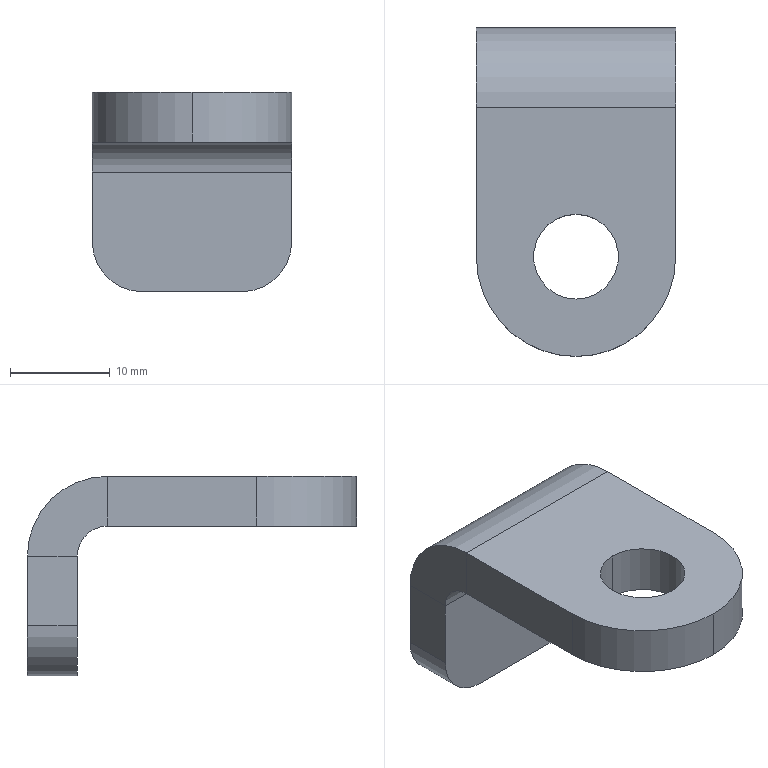Part | SolidWorks | features Fillet 2, FlatPattern 1, ICE 1, SMBaseFlange 1, SheetMetal 1 | 1 solid | 19 faces | box 20 x 33 x 20 mm | volume 4012 mm3 | plane 11 | cylinder 8 | commonest cylinder face diameters 8.5 x2 10 x2 20 x2 6 x1 16 x1
STEP:
#1=CARTESIAN_POINT('',(10.,-18.75,0.));
#2=VERTEX_POINT('',#1);
#3=CARTESIAN_POINT('',(10.,-27.25,0.));
#4=VERTEX_POINT('',#3);
#5=CARTESIAN_POINT('',(10.,-23.,0.));
#6=DIRECTION('',(0.,0.,1.));
#7=DIRECTION('',(0.,1.,0.));
#8=AXIS2_PLACEMENT_3D('',#5,#6,#7);
#9=CIRCLE('',#8,4.25);
#10=EDGE_CURVE('',#2,#4,#9,.T.);
#11=ORIENTED_EDGE('',*,*,#10,.T.);
#12=CARTESIAN_POINT('',(10.,-27.25,-5.));
#13=VERTEX_POINT('',#12);
#14=CARTESIAN_POINT('',(10.,-27.25,0.001));
#15=DIRECTION('',(0.,0.,-1.));
#16=VECTOR('',#15,1000.);
#17=LINE('',#14,#16);
#18=EDGE_CURVE('',#4,#13,#17,.T.);
#19=ORIENTED_EDGE('',*,*,#18,.T.);
#20=CARTESIAN_POINT('',(10.,-18.75,-5.));
#21=VERTEX_POINT('',#20);
#22=CARTESIAN_POINT('',(10.,-23.,-5.));
#23=DIRECTION('',(0.,0.,-1.));
#24=DIRECTION('',(0.,1.,0.));
#25=AXIS2_PLACEMENT_3D('',#22,#23,#24);
#26=CIRCLE('',#25,4.25);
#27=EDGE_CURVE('',#13,#21,#26,.T.);
#28=ORIENTED_EDGE('',*,*,#27,.T.);
#29=CARTESIAN_POINT('',(10.,-18.75,0.001));
#30=DIRECTION('',(0.,0.,-1.));
#31=VECTOR('',#30,1000.);
#32=LINE('',#29,#31);
#33=EDGE_CURVE('',#2,#21,#32,.T.);
#34=ORIENTED_EDGE('',*,*,#33,.F.);
#35=EDGE_LOOP('',(#11,#19,#28,#34));
#36=FACE_OUTER_BOUND('',#35,.T.);
#37=CARTESIAN_POINT('',(10.,-23.,0.001));
#38=DIRECTION('',(0.,0.,-1.));
#39=DIRECTION('',(0.,1.,0.));
#40=AXIS2_PLACEMENT_3D('',#37,#38,#39);
#41=CYLINDRICAL_SURFACE('',#40,4.25);
#42=ADVANCED_FACE('',(#36),#41,.F.);
#43=CARTESIAN_POINT('',(20.,0.,-8.));
#44=VERTEX_POINT('',#43);
#45=CARTESIAN_POINT('',(20.,-5.,-8.));
#46=VERTEX_POINT('',#45);
#47=CARTESIAN_POINT('',(20.,0.,-8.));
#48=DIRECTION('',(0.,-1.,0.));
#49=VECTOR('',#48,1000.);
#50=LINE('',#47,#49);
#51=EDGE_CURVE('',#44,#46,#50,.T.);
#52=ORIENTED_EDGE('',*,*,#51,.F.);
#53=CARTESIAN_POINT('',(20.,-8.,0.));
#54=VERTEX_POINT('',#53);
#55=CARTESIAN_POINT('',(20.,-8.,-8.));
#56=DIRECTION('',(1.,0.,0.));
#57=DIRECTION('',(0.,0.,1.));
#58=AXIS2_PLACEMENT_3D('',#55,#56,#57);
#59=CIRCLE('',#58,8.);
#60=EDGE_CURVE('',#44,#54,#59,.T.);
#61=ORIENTED_EDGE('',*,*,#60,.T.);
#62=CARTESIAN_POINT('',(20.,-8.,-5.));
#63=VERTEX_POINT('',#62);
#64=CARTESIAN_POINT('',(20.,-8.,-5.));
#65=DIRECTION('',(0.,0.,1.));
#66=VECTOR('',#65,1000.);
#67=LINE('',#64,#66);
#68=EDGE_CURVE('',#63,#54,#67,.T.);
#69=ORIENTED_EDGE('',*,*,#68,.F.);
#70=CARTESIAN_POINT('',(20.,-8.,-8.));
#71=DIRECTION('',(1.,0.,0.));
#72=DIRECTION('',(0.,0.,-1.));
#73=AXIS2_PLACEMENT_3D('',#70,#71,#72);
#74=CIRCLE('',#73,3.);
#75=EDGE_CURVE('',#46,#63,#74,.T.);
#76=ORIENTED_EDGE('',*,*,#75,.F.);
#77=EDGE_LOOP('',(#52,#61,#69,#76));
#78=FACE_OUTER_BOUND('',#77,.T.);
#79=CARTESIAN_POINT('',(20.,0.,-8.));
#80=DIRECTION('',(1.,0.,0.));
#81=DIRECTION('',(0.,0.,-1.));
#82=AXIS2_PLACEMENT_3D('',#79,#80,#81);
#83=PLANE('',#82);
#84=ADVANCED_FACE('',(#78),#83,.T.);
#85=CARTESIAN_POINT('',(20.,-5.,-15.));
#86=VERTEX_POINT('',#85);
#87=CARTESIAN_POINT('',(20.,-5.,0.));
#88=DIRECTION('',(0.,0.,1.));
#89=VECTOR('',#88,1000.);
#90=LINE('',#87,#89);
#91=EDGE_CURVE('',#86,#46,#90,.T.);
#92=ORIENTED_EDGE('',*,*,#91,.F.);
#93=CARTESIAN_POINT('',(20.,0.,-15.));
#94=VERTEX_POINT('',#93);
#95=CARTESIAN_POINT('',(20.,-8.,-15.));
#96=DIRECTION('',(0.,1.,0.));
#97=VECTOR('',#96,1000.);
#98=LINE('',#95,#97);
#99=EDGE_CURVE('',#86,#94,#98,.T.);
#100=ORIENTED_EDGE('',*,*,#99,.T.);
#101=CARTESIAN_POINT('',(20.,0.,0.));
#102=DIRECTION('',(0.,0.,1.));
#103=VECTOR('',#102,1000.);
#104=LINE('',#101,#103);
#105=EDGE_CURVE('',#94,#44,#104,.T.);
#106=ORIENTED_EDGE('',*,*,#105,.T.);
#107=ORIENTED_EDGE('',*,*,#51,.T.);
#108=EDGE_LOOP('',(#92,#100,#106,#107));
#109=FACE_OUTER_BOUND('',#108,.T.);
#110=CARTESIAN_POINT('',(20.,-8.,-5.));
#111=DIRECTION('',(1.,0.,0.));
#112=DIRECTION('',(0.,0.,-1.));
#113=AXIS2_PLACEMENT_3D('',#110,#111,#112);
#114=PLANE('',#113);
#115=ADVANCED_FACE('',(#109),#114,.T.);
#116=CARTESIAN_POINT('',(0.,-8.,0.));
#117=VERTEX_POINT('',#116);
#118=CARTESIAN_POINT('',(0.,-8.,-5.));
#119=VERTEX_POINT('',#118);
#120=CARTESIAN_POINT('',(0.,-8.,0.));
#121=DIRECTION('',(0.,0.,-1.));
#122=VECTOR('',#121,1000.);
#123=LINE('',#120,#122);
#124=EDGE_CURVE('',#117,#119,#123,.T.);
#125=ORIENTED_EDGE('',*,*,#124,.F.);
#126=CARTESIAN_POINT('',(0.,0.,-8.));
#127=VERTEX_POINT('',#126);
#128=CARTESIAN_POINT('',(0.,-8.,-8.));
#129=DIRECTION('',(1.,0.,0.));
#130=DIRECTION('',(0.,0.,1.));
#131=AXIS2_PLACEMENT_3D('',#128,#129,#130);
#132=CIRCLE('',#131,8.);
#133=EDGE_CURVE('',#127,#117,#132,.T.);
#134=ORIENTED_EDGE('',*,*,#133,.F.);
#135=CARTESIAN_POINT('',(0.,-5.,-8.));
#136=VERTEX_POINT('',#135);
#137=CARTESIAN_POINT('',(0.,-5.,-8.));
#138=DIRECTION('',(0.,1.,0.));
#139=VECTOR('',#138,1000.);
#140=LINE('',#137,#139);
#141=EDGE_CURVE('',#136,#127,#140,.T.);
#142=ORIENTED_EDGE('',*,*,#141,.F.);
#143=CARTESIAN_POINT('',(0.,-8.,-8.));
#144=DIRECTION('',(1.,0.,0.));
#145=DIRECTION('',(0.,0.,-1.));
#146=AXIS2_PLACEMENT_3D('',#143,#144,#145);
#147=CIRCLE('',#146,3.);
#148=EDGE_CURVE('',#136,#119,#147,.T.);
#149=ORIENTED_EDGE('',*,*,#148,.T.);
#150=EDGE_LOOP('',(#125,#134,#142,#149));
#151=FACE_OUTER_BOUND('',#150,.T.);
#152=CARTESIAN_POINT('',(0.,-8.,0.));
#153=DIRECTION('',(-1.,0.,0.));
#154=DIRECTION('',(0.,0.,1.));
#155=AXIS2_PLACEMENT_3D('',#152,#153,#154);
#156=PLANE('',#155);
#157=ADVANCED_FACE('',(#151),#156,.T.);
#158=CARTESIAN_POINT('',(0.,-23.,-5.));
#159=VERTEX_POINT('',#158);
#160=CARTESIAN_POINT('',(0.,0.,-5.));
#161=DIRECTION('',(0.,-1.,0.));
#162=VECTOR('',#161,1000.);
#163=LINE('',#160,#162);
#164=EDGE_CURVE('',#119,#159,#163,.T.);
#165=ORIENTED_EDGE('',*,*,#164,.T.);
#166=CARTESIAN_POINT('',(0.,-23.,0.));
#167=VERTEX_POINT('',#166);
#168=CARTESIAN_POINT('',(0.,-23.,-8.));
#169=DIRECTION('',(0.,0.,1.));
#170=VECTOR('',#169,1000.);
#171=LINE('',#168,#170);
#172=EDGE_CURVE('',#159,#167,#171,.T.);
#173=ORIENTED_EDGE('',*,*,#172,.T.);
#174=CARTESIAN_POINT('',(0.,0.,0.));
#175=DIRECTION('',(0.,-1.,0.));
#176=VECTOR('',#175,1000.);
#177=LINE('',#174,#176);
#178=EDGE_CURVE('',#117,#167,#177,.T.);
#179=ORIENTED_EDGE('',*,*,#178,.F.);
#180=ORIENTED_EDGE('',*,*,#124,.T.);
#181=EDGE_LOOP('',(#165,#173,#179,#180));
#182=FACE_OUTER_BOUND('',#181,.T.);
#183=CARTESIAN_POINT('',(0.,-5.,-8.));
#184=DIRECTION('',(-1.,0.,0.));
#185=DIRECTION('',(0.,0.,1.));
#186=AXIS2_PLACEMENT_3D('',#183,#184,#185);
#187=PLANE('',#186);
#188=ADVANCED_FACE('',(#182),#187,.T.);
#189=ORIENTED_EDGE('',*,*,#10,.F.);
#190=CARTESIAN_POINT('',(10.,-23.,0.));
#191=DIRECTION('',(0.,0.,1.));
#192=DIRECTION('',(0.,1.,0.));
#193=AXIS2_PLACEMENT_3D('',#190,#191,#192);
#194=CIRCLE('',#193,4.25);
#195=EDGE_CURVE('',#4,#2,#194,.T.);
#196=ORIENTED_EDGE('',*,*,#195,.F.);
#197=EDGE_LOOP('',(#189,#196));
#198=FACE_BOUND('',#197,.T.);
#199=ORIENTED_EDGE('',*,*,#178,.T.);
#200=CARTESIAN_POINT('',(10.,-33.,0.));
#201=VERTEX_POINT('',#200);
#202=CARTESIAN_POINT('',(10.,-23.,0.));
#203=DIRECTION('',(0.,0.,1.));
#204=DIRECTION('',(0.,1.,0.));
#205=AXIS2_PLACEMENT_3D('',#202,#203,#204);
#206=CIRCLE('',#205,10.);
#207=EDGE_CURVE('',#167,#201,#206,.T.);
#208=ORIENTED_EDGE('',*,*,#207,.T.);
#209=CARTESIAN_POINT('',(20.,-23.,0.));
#210=VERTEX_POINT('',#209);
#211=CARTESIAN_POINT('',(10.,-23.,0.));
#212=DIRECTION('',(0.,0.,1.));
#213=DIRECTION('',(0.,1.,0.));
#214=AXIS2_PLACEMENT_3D('',#211,#212,#213);
#215=CIRCLE('',#214,10.);
#216=EDGE_CURVE('',#201,#210,#215,.T.);
#217=ORIENTED_EDGE('',*,*,#216,.T.);
#218=CARTESIAN_POINT('',(20.,0.,0.));
#219=DIRECTION('',(0.,-1.,0.));
#220=VECTOR('',#219,1000.);
#221=LINE('',#218,#220);
#222=EDGE_CURVE('',#54,#210,#221,.T.);
#223=ORIENTED_EDGE('',*,*,#222,.F.);
#224=CARTESIAN_POINT('',(20.,-8.,0.));
#225=DIRECTION('',(-1.,0.,0.));
#226=VECTOR('',#225,1000.);
#227=LINE('',#224,#226);
#228=EDGE_CURVE('',#54,#117,#227,.T.);
#229=ORIENTED_EDGE('',*,*,#228,.T.);
#230=EDGE_LOOP('',(#199,#208,#217,#223,#229));
#231=FACE_OUTER_BOUND('',#230,.T.);
#232=CARTESIAN_POINT('',(20.,0.,0.));
#233=DIRECTION('',(0.,0.,-1.));
#234=DIRECTION('',(0.,1.,0.));
#235=AXIS2_PLACEMENT_3D('',#232,#233,#234);
#236=PLANE('',#235);
#237=ADVANCED_FACE('',(#198,#231),#236,.F.);
#238=CARTESIAN_POINT('',(10.,-23.,-5.));
#239=DIRECTION('',(0.,0.,-1.));
#240=DIRECTION('',(0.,1.,0.));
#241=AXIS2_PLACEMENT_3D('',#238,#239,#240);
#242=CIRCLE('',#241,4.25);
#243=EDGE_CURVE('',#21,#13,#242,.T.);
#244=ORIENTED_EDGE('',*,*,#243,.F.);
#245=ORIENTED_EDGE('',*,*,#27,.F.);
#246=EDGE_LOOP('',(#244,#245));
#247=FACE_BOUND('',#246,.T.);
#248=CARTESIAN_POINT('',(20.,-23.,-5.));
#249=VERTEX_POINT('',#248);
#250=CARTESIAN_POINT('',(10.,-33.,-5.));
#251=VERTEX_POINT('',#250);
#252=CARTESIAN_POINT('',(10.,-23.,-5.));
#253=DIRECTION('',(0.,0.,-1.));
#254=DIRECTION('',(0.,1.,0.));
#255=AXIS2_PLACEMENT_3D('',#252,#253,#254);
#256=CIRCLE('',#255,10.);
#257=EDGE_CURVE('',#249,#251,#256,.T.);
#258=ORIENTED_EDGE('',*,*,#257,.T.);
#259=CARTESIAN_POINT('',(10.,-23.,-5.));
#260=DIRECTION('',(0.,0.,-1.));
#261=DIRECTION('',(0.,1.,0.));
#262=AXIS2_PLACEMENT_3D('',#259,#260,#261);
#263=CIRCLE('',#262,10.);
#264=EDGE_CURVE('',#251,#159,#263,.T.);
#265=ORIENTED_EDGE('',*,*,#264,.T.);
#266=ORIENTED_EDGE('',*,*,#164,.F.);
#267=CARTESIAN_POINT('',(20.,-8.,-5.));
#268=DIRECTION('',(-1.,0.,0.));
#269=VECTOR('',#268,1000.);
#270=LINE('',#267,#269);
#271=EDGE_CURVE('',#63,#119,#270,.T.);
#272=ORIENTED_EDGE('',*,*,#271,.F.);
#273=CARTESIAN_POINT('',(20.,0.,-5.));
#274=DIRECTION('',(0.,-1.,0.));
#275=VECTOR('',#274,1000.);
#276=LINE('',#273,#275);
#277=EDGE_CURVE('',#63,#249,#276,.T.);
#278=ORIENTED_EDGE('',*,*,#277,.T.);
#279=EDGE_LOOP('',(#258,#265,#266,#272,#278));
#280=FACE_OUTER_BOUND('',#279,.T.);
#281=CARTESIAN_POINT('',(20.,0.,-5.));
#282=DIRECTION('',(0.,0.,-1.));
#283=DIRECTION('',(0.,1.,0.));
#284=AXIS2_PLACEMENT_3D('',#281,#282,#283);
#285=PLANE('',#284);
#286=ADVANCED_FACE('',(#247,#280),#285,.T.);
#287=ORIENTED_EDGE('',*,*,#148,.F.);
#288=CARTESIAN_POINT('',(20.,-5.,-8.));
#289=DIRECTION('',(-1.,0.,0.));
#290=VECTOR('',#289,1000.);
#291=LINE('',#288,#290);
#292=EDGE_CURVE('',#46,#136,#291,.T.);
#293=ORIENTED_EDGE('',*,*,#292,.F.);
#294=ORIENTED_EDGE('',*,*,#75,.T.);
#295=ORIENTED_EDGE('',*,*,#271,.T.);
#296=EDGE_LOOP('',(#287,#293,#294,#295));
#297=FACE_OUTER_BOUND('',#296,.T.);
#298=CARTESIAN_POINT('',(20.,-8.,-8.));
#299=DIRECTION('',(-1.,0.,0.));
#300=DIRECTION('',(0.,0.,1.));
#301=AXIS2_PLACEMENT_3D('',#298,#299,#300);
#302=CYLINDRICAL_SURFACE('',#301,3.);
#303=ADVANCED_FACE('',(#297),#302,.F.);
#304=CARTESIAN_POINT('',(0.,-5.,-15.));
#305=VERTEX_POINT('',#304);
#306=CARTESIAN_POINT('',(0.,-5.,0.));
#307=DIRECTION('',(0.,0.,1.));
#308=VECTOR('',#307,1000.);
#309=LINE('',#306,#308);
#310=EDGE_CURVE('',#305,#136,#309,.T.);
#311=ORIENTED_EDGE('',*,*,#310,.F.);
#312=CARTESIAN_POINT('',(5.,-5.,-20.));
#313=VERTEX_POINT('',#312);
#314=CARTESIAN_POINT('',(5.,-5.,-15.));
#315=DIRECTION('',(0.,-1.,0.));
#316=DIRECTION('',(0.,0.,-1.));
#317=AXIS2_PLACEMENT_3D('',#314,#315,#316);
#318=CIRCLE('',#317,5.);
#319=EDGE_CURVE('',#305,#313,#318,.T.);
#320=ORIENTED_EDGE('',*,*,#319,.T.);
#321=CARTESIAN_POINT('',(15.,-5.,-20.));
#322=VERTEX_POINT('',#321);
#323=CARTESIAN_POINT('',(20.,-5.,-20.));
#324=DIRECTION('',(-1.,0.,0.));
#325=VECTOR('',#324,1000.);
#326=LINE('',#323,#325);
#327=EDGE_CURVE('',#322,#313,#326,.T.);
#328=ORIENTED_EDGE('',*,*,#327,.F.);
#329=CARTESIAN_POINT('',(15.,-5.,-15.));
#330=DIRECTION('',(0.,-1.,0.));
#331=DIRECTION('',(0.,0.,-1.));
#332=AXIS2_PLACEMENT_3D('',#329,#330,#331);
#333=CIRCLE('',#332,5.);
#334=EDGE_CURVE('',#322,#86,#333,.T.);
#335=ORIENTED_EDGE('',*,*,#334,.T.);
#336=ORIENTED_EDGE('',*,*,#91,.T.);
#337=ORIENTED_EDGE('',*,*,#292,.T.);
#338=EDGE_LOOP('',(#311,#320,#328,#335,#336,#337));
#339=FACE_OUTER_BOUND('',#338,.T.);
#340=CARTESIAN_POINT('',(20.,-5.,0.));
#341=DIRECTION('',(0.,-1.,0.));
#342=DIRECTION('',(0.,0.,-1.));
#343=AXIS2_PLACEMENT_3D('',#340,#341,#342);
#344=PLANE('',#343);
#345=ADVANCED_FACE('',(#339),#344,.T.);
#346=ORIENTED_EDGE('',*,*,#327,.T.);
#347=CARTESIAN_POINT('',(5.,0.,-20.));
#348=VERTEX_POINT('',#347);
#349=CARTESIAN_POINT('',(5.,0.,-20.));
#350=DIRECTION('',(0.,1.,0.));
#351=VECTOR('',#350,1000.);
#352=LINE('',#349,#351);
#353=EDGE_CURVE('',#313,#348,#352,.T.);
#354=ORIENTED_EDGE('',*,*,#353,.T.);
#355=CARTESIAN_POINT('',(15.,0.,-20.));
#356=VERTEX_POINT('',#355);
#357=CARTESIAN_POINT('',(20.,0.,-20.));
#358=DIRECTION('',(-1.,0.,0.));
#359=VECTOR('',#358,1000.);
#360=LINE('',#357,#359);
#361=EDGE_CURVE('',#356,#348,#360,.T.);
#362=ORIENTED_EDGE('',*,*,#361,.F.);
#363=CARTESIAN_POINT('',(15.,0.,-20.));
#364=DIRECTION('',(0.,-1.,0.));
#365=VECTOR('',#364,1000.);
#366=LINE('',#363,#365);
#367=EDGE_CURVE('',#356,#322,#366,.T.);
#368=ORIENTED_EDGE('',*,*,#367,.T.);
#369=EDGE_LOOP('',(#346,#354,#362,#368));
#370=FACE_OUTER_BOUND('',#369,.T.);
#371=CARTESIAN_POINT('',(20.,0.,-20.));
#372=DIRECTION('',(0.,0.,-1.));
#373=DIRECTION('',(-1.,0.,0.));
#374=AXIS2_PLACEMENT_3D('',#371,#372,#373);
#375=PLANE('',#374);
#376=ADVANCED_FACE('',(#370),#375,.T.);
#377=ORIENTED_EDGE('',*,*,#361,.T.);
#378=CARTESIAN_POINT('',(0.,0.,-15.));
#379=VERTEX_POINT('',#378);
#380=CARTESIAN_POINT('',(5.,0.,-15.));
#381=DIRECTION('',(0.,1.,0.));
#382=DIRECTION('',(0.,0.,-1.));
#383=AXIS2_PLACEMENT_3D('',#380,#381,#382);
#384=CIRCLE('',#383,5.);
#385=EDGE_CURVE('',#348,#379,#384,.T.);
#386=ORIENTED_EDGE('',*,*,#385,.T.);
#387=CARTESIAN_POINT('',(0.,0.,0.));
#388=DIRECTION('',(0.,0.,1.));
#389=VECTOR('',#388,1000.);
#390=LINE('',#387,#389);
#391=EDGE_CURVE('',#379,#127,#390,.T.);
#392=ORIENTED_EDGE('',*,*,#391,.T.);
#393=CARTESIAN_POINT('',(20.,0.,-8.));
#394=DIRECTION('',(-1.,0.,0.));
#395=VECTOR('',#394,1000.);
#396=LINE('',#393,#395);
#397=EDGE_CURVE('',#44,#127,#396,.T.);
#398=ORIENTED_EDGE('',*,*,#397,.F.);
#399=ORIENTED_EDGE('',*,*,#105,.F.);
#400=CARTESIAN_POINT('',(15.,0.,-15.));
#401=DIRECTION('',(0.,1.,0.));
#402=DIRECTION('',(0.,0.,-1.));
#403=AXIS2_PLACEMENT_3D('',#400,#401,#402);
#404=CIRCLE('',#403,5.);
#405=EDGE_CURVE('',#94,#356,#404,.T.);
#406=ORIENTED_EDGE('',*,*,#405,.T.);
#407=EDGE_LOOP('',(#377,#386,#392,#398,#399,#406));
#408=FACE_OUTER_BOUND('',#407,.T.);
#409=CARTESIAN_POINT('',(20.,0.,0.));
#410=DIRECTION('',(0.,-1.,0.));
#411=DIRECTION('',(0.,0.,-1.));
#412=AXIS2_PLACEMENT_3D('',#409,#410,#411);
#413=PLANE('',#412);
#414=ADVANCED_FACE('',(#408),#413,.F.);
#415=ORIENTED_EDGE('',*,*,#133,.T.);
#416=ORIENTED_EDGE('',*,*,#228,.F.);
#417=ORIENTED_EDGE('',*,*,#60,.F.);
#418=ORIENTED_EDGE('',*,*,#397,.T.);
#419=EDGE_LOOP('',(#415,#416,#417,#418));
#420=FACE_OUTER_BOUND('',#419,.T.);
#421=CARTESIAN_POINT('',(20.,-8.,-8.));
#422=DIRECTION('',(-1.,0.,0.));
#423=DIRECTION('',(0.,0.,1.));
#424=AXIS2_PLACEMENT_3D('',#421,#422,#423);
#425=CYLINDRICAL_SURFACE('',#424,8.);
#426=ADVANCED_FACE('',(#420),#425,.T.);
#427=ORIENTED_EDGE('',*,*,#222,.T.);
#428=CARTESIAN_POINT('',(20.,-23.,-8.));
#429=DIRECTION('',(0.,0.,-1.));
#430=VECTOR('',#429,1000.);
#431=LINE('',#428,#430);
#432=EDGE_CURVE('',#210,#249,#431,.T.);
#433=ORIENTED_EDGE('',*,*,#432,.T.);
#434=ORIENTED_EDGE('',*,*,#277,.F.);
#435=ORIENTED_EDGE('',*,*,#68,.T.);
#436=EDGE_LOOP('',(#427,#433,#434,#435));
#437=FACE_OUTER_BOUND('',#436,.T.);
#438=CARTESIAN_POINT('',(20.,-8.,-8.));
#439=DIRECTION('',(1.,0.,0.));
#440=DIRECTION('',(0.,0.,-1.));
#441=AXIS2_PLACEMENT_3D('',#438,#439,#440);
#442=PLANE('',#441);
#443=ADVANCED_FACE('',(#437),#442,.T.);
#444=ORIENTED_EDGE('',*,*,#391,.F.);
#445=CARTESIAN_POINT('',(0.,-5.,-15.));
#446=DIRECTION('',(0.,-1.,0.));
#447=VECTOR('',#446,1000.);
#448=LINE('',#445,#447);
#449=EDGE_CURVE('',#379,#305,#448,.T.);
#450=ORIENTED_EDGE('',*,*,#449,.T.);
#451=ORIENTED_EDGE('',*,*,#310,.T.);
#452=ORIENTED_EDGE('',*,*,#141,.T.);
#453=EDGE_LOOP('',(#444,#450,#451,#452));
#454=FACE_OUTER_BOUND('',#453,.T.);
#455=CARTESIAN_POINT('',(0.,-8.,-8.));
#456=DIRECTION('',(1.,0.,0.));
#457=DIRECTION('',(0.,0.,-1.));
#458=AXIS2_PLACEMENT_3D('',#455,#456,#457);
#459=PLANE('',#458);
#460=ADVANCED_FACE('',(#454),#459,.F.);
#461=CARTESIAN_POINT('',(10.,-33.,-5.));
#462=DIRECTION('',(0.,0.,1.));
#463=VECTOR('',#462,1000.);
#464=LINE('',#461,#463);
#465=EDGE_CURVE('',#251,#201,#464,.T.);
#466=ORIENTED_EDGE('',*,*,#465,.F.);
#467=ORIENTED_EDGE('',*,*,#257,.F.);
#468=ORIENTED_EDGE('',*,*,#432,.F.);
#469=ORIENTED_EDGE('',*,*,#216,.F.);
#470=EDGE_LOOP('',(#466,#467,#468,#469));
#471=FACE_OUTER_BOUND('',#470,.T.);
#472=CARTESIAN_POINT('',(10.,-23.,-5.));
#473=DIRECTION('',(0.,0.,1.));
#474=DIRECTION('',(1.,0.,0.));
#475=AXIS2_PLACEMENT_3D('',#472,#473,#474);
#476=CYLINDRICAL_SURFACE('',#475,10.);
#477=ADVANCED_FACE('',(#471),#476,.T.);
#478=ORIENTED_EDGE('',*,*,#264,.F.);
#479=ORIENTED_EDGE('',*,*,#465,.T.);
#480=ORIENTED_EDGE('',*,*,#207,.F.);
#481=ORIENTED_EDGE('',*,*,#172,.F.);
#482=EDGE_LOOP('',(#478,#479,#480,#481));
#483=FACE_OUTER_BOUND('',#482,.T.);
#484=CARTESIAN_POINT('',(10.,-23.,-8.));
#485=DIRECTION('',(0.,0.,1.));
#486=DIRECTION('',(1.,0.,0.));
#487=AXIS2_PLACEMENT_3D('',#484,#485,#486);
#488=CYLINDRICAL_SURFACE('',#487,10.);
#489=ADVANCED_FACE('',(#483),#488,.T.);
#490=ORIENTED_EDGE('',*,*,#385,.F.);
#491=ORIENTED_EDGE('',*,*,#353,.F.);
#492=ORIENTED_EDGE('',*,*,#319,.F.);
#493=ORIENTED_EDGE('',*,*,#449,.F.);
#494=EDGE_LOOP('',(#490,#491,#492,#493));
#495=FACE_OUTER_BOUND('',#494,.T.);
#496=CARTESIAN_POINT('',(5.,-8.,-15.));
#497=DIRECTION('',(0.,1.,0.));
#498=DIRECTION('',(0.,0.,1.));
#499=AXIS2_PLACEMENT_3D('',#496,#497,#498);
#500=CYLINDRICAL_SURFACE('',#499,5.);
#501=ADVANCED_FACE('',(#495),#500,.T.);
#502=ORIENTED_EDGE('',*,*,#405,.F.);
#503=ORIENTED_EDGE('',*,*,#99,.F.);
#504=ORIENTED_EDGE('',*,*,#334,.F.);
#505=ORIENTED_EDGE('',*,*,#367,.F.);
#506=EDGE_LOOP('',(#502,#503,#504,#505));
#507=FACE_OUTER_BOUND('',#506,.T.);
#508=CARTESIAN_POINT('',(15.,0.,-15.));
#509=DIRECTION('',(0.,-1.,0.));
#510=DIRECTION('',(0.,0.,-1.));
#511=AXIS2_PLACEMENT_3D('',#508,#509,#510);
#512=CYLINDRICAL_SURFACE('',#511,5.);
#513=ADVANCED_FACE('',(#507),#512,.T.);
#514=ORIENTED_EDGE('',*,*,#18,.F.);
#515=ORIENTED_EDGE('',*,*,#195,.T.);
#516=ORIENTED_EDGE('',*,*,#33,.T.);
#517=ORIENTED_EDGE('',*,*,#243,.T.);
#518=EDGE_LOOP('',(#514,#515,#516,#517));
#519=FACE_OUTER_BOUND('',#518,.T.);
#520=CARTESIAN_POINT('',(10.,-23.,0.001));
#521=DIRECTION('',(0.,0.,-1.));
#522=DIRECTION('',(0.,1.,0.));
#523=AXIS2_PLACEMENT_3D('',#520,#521,#522);
#524=CYLINDRICAL_SURFACE('',#523,4.25);
#525=ADVANCED_FACE('',(#519),#524,.F.);
#526=CLOSED_SHELL('',(#42,#84,#115,#157,#188,#237,#286,#303,#345,#376,#414,#426,#443,#460,#477,#489,#501,#513,#525));
#527=MANIFOLD_SOLID_BREP('',#526);
#528=CARTESIAN_POINT('',(0.,0.,0.));
#529=DIRECTION('',(0.,0.,1.));
#530=DIRECTION('',(1.,0.,0.));
#531=AXIS2_PLACEMENT_3D('',#528,#529,#530);
#532=(LENGTH_UNIT()NAMED_UNIT(*)SI_UNIT(.MILLI.,.METRE.));
#533=UNCERTAINTY_MEASURE_WITH_UNIT(LENGTH_MEASURE(0.00001),#532,'','');
#534=(NAMED_UNIT(*)PLANE_ANGLE_UNIT()SI_UNIT($,.RADIAN.));
#535=(NAMED_UNIT(*)SI_UNIT($,.STERADIAN.)SOLID_ANGLE_UNIT());
#536=(GEOMETRIC_REPRESENTATION_CONTEXT(3)GLOBAL_UNCERTAINTY_ASSIGNED_CONTEXT((#533))GLOBAL_UNIT_ASSIGNED_CONTEXT((#532,#534,#535))REPRESENTATION_CONTEXT('',''));
#537=ADVANCED_BREP_SHAPE_REPRESENTATION('',(#527,#531),#536);